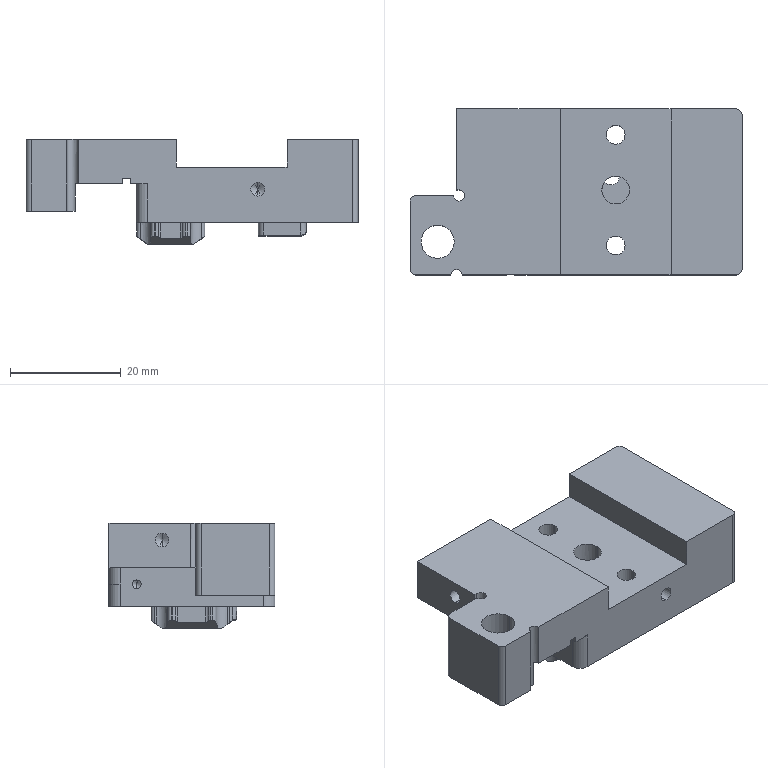Part | STEP file | 06-02-01 rotary fixture | 1 solid | 141 faces | box 60 x 30 x 19 mm | volume 18912 mm3 | cylinder 74 | plane 57 | cone 6 | spline 4 | commonest cylinder face diameters 1.2 x16 2 x11 3 x11 1 x8 4 x7 6 x6